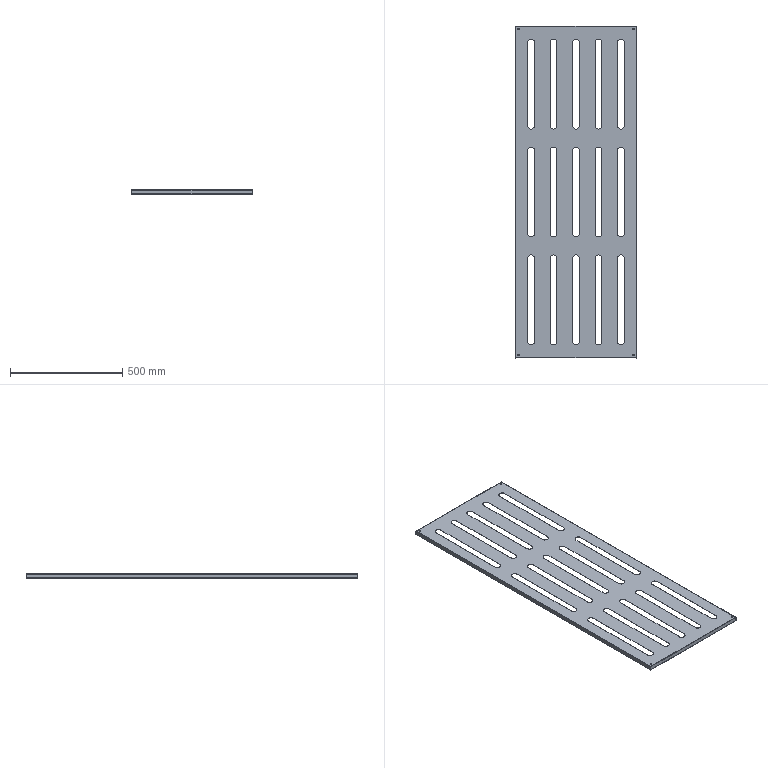Part | STEP file | 1 solid | 140 faces | box 537 x 1477 x 19.5 mm | volume 715905 mm3 | plane 86 | cylinder 54 | commonest cylinder face diameters 30 x30 0.4 x8 2.4 x8 6 x8